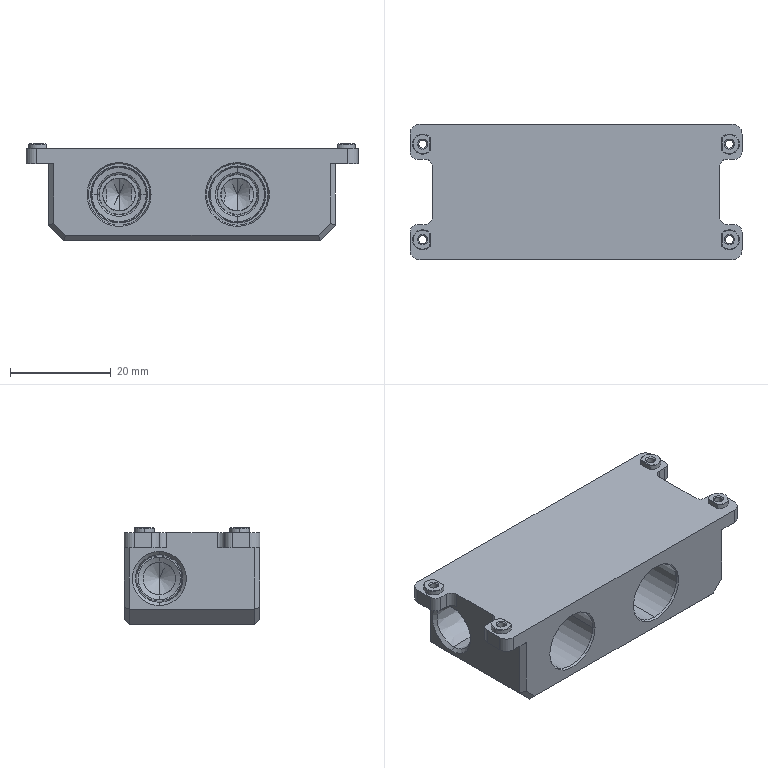NC program | NX | posted with a generic post | part box 66 x 27 x 19.25 mm
Lines 4327 to 5134 of 6448:
(DRILLING_1 , TOOL : D3倒角刀)
N8598 T05 M6
N8600 G54
N8602 G17 G0 G90 X-6.5 Y9.125 S2000 M3
N8604 G43 Z15.5 H5
N8606 G94 G81 G99 Z-5.5 F200. R-1.5
N8608 G80
N8610 G0 X-6.5 Y9.125 Z15.5
N8612 M5
(DRILLING_6 , TOOL : D6.5钻头)
N8614 T09 M6
N8616 G54
N8618 G17 G0 G90 X-6.5 Y9.125 S2000 M3
N8620 G43 Z15.5 H9
N8622 G94 G81 G98 Z-50.5 F200. R-1.5
N8624 G80
N8626 G0 X-6.5 Y9.125 Z15.5
N8628 M5
(DRILLING_2 , TOOL : D8.4钻头)
N8630 T10 M6
N8632 G54
N8634 G17 G0 G90 X-6.5 Y9.125 S1600 M3
N8636 G43 Z15.5 H10
N8638 G94 G83 G98 Z-16.5 F200. Q3. R-1.5
N8640 G80
N8642 G0 X-6.5 Y9.125 Z15.5
N8644 M5
(PLANAR_MILL_4 , TOOL : D3倒角刀)
N8646 T05 M6
N8648 G54
N8650 G17 G0 G90 X-7.5 Y6.038 S4500 M3
N8652 G43 Z15.5 H5
N8654 Z-3.5
N8656 G94 G1 Z-5.5 F600.
N8658 Y5.88
N8660 G3 X-6.5 Y4.88 R1.
N8662 X-2.255 Y9.125 R4.245
N8664 X-6.5 Y4.88 R-4.245
N8666 X-5.5 Y5.88 R1.
N8668 G1 Y6.038
N8670 Z-3.5
N8672 G0 Z15.5
N8674 M5
(THREAD_MILLING , TOOL : NPT)
N8676 T11 M6
N8678 G54
N8680 G17 G0 G90 X-6.5 Y9.125 S4500 M3
N8682 G43 Z15.5 H11
N8684 Z-11.547
N8686 G41 G94 G1 X-6.024 Y8.972 F300. D11
N8688 G3 X-5.595 Y9.555 Z-11.42 R0.412
N8690 X-6.143 Y10.065 Z-11.31 R1.003
N8692 X-6.895 Y10.053 Z-11.199 R1.008
N8694 X-7.43 Y9.524 Z-11.089 R1.01
N8696 X-7.45 Y8.767 Z-10.978 R1.014
N8698 X-6.94 Y8.206 Z-10.868 R1.017
N8700 X-6.18 Y8.154 Z-10.758 R1.021
N8702 X-5.594 Y8.644 Z-10.648 R1.024
N8704 X-5.51 Y9.407 Z-10.537 R1.028
N8706 X-5.979 Y10.017 Z-10.427 R1.031
N8708 X-6.742 Y10.133 Z-10.316 R1.035
N8710 X-7.375 Y9.687 Z-10.206 R1.037
N8712 X-7.524 Y8.924 Z-10.095 R1.042
N8714 X-7.102 Y8.268 Z-9.985 R1.044
N8716 X-6.34 Y8.087 Z-9.875 R1.049
N8718 X-5.664 Y8.484 Z-9.765 R1.051
N8720 X-5.45 Y9.242 Z-9.654 R1.056
N8722 X-5.821 Y9.939 Z-9.544 R1.058
N8724 X-6.574 Y10.186 Z-9.433 R1.063
N8726 X-7.29 Y9.842 Z-9.323 R1.065
N8728 X-7.57 Y9.095 Z-9.212 R1.07
N8730 X-7.254 Y8.36 Z-9.102 R1.072
N8732 X-6.514 Y8.047 Z-8.992 R1.077
N8734 X-5.762 Y8.335 Z-8.882 R1.079
N8736 X-5.417 Y9.066 Z-8.771 R1.083
N8738 X-5.674 Y9.834 Z-8.661 R1.086
N8740 X-6.395 Y10.211 Z-8.55 R1.09
N8742 X-7.178 Y9.985 Z-8.44 R1.093
N8744 X-7.588 Y9.276 Z-8.329 R1.097
N8746 X-7.393 Y8.479 Z-8.219 R1.1
N8748 X-6.697 Y8.037 Z-8.109 R1.104
N8750 X-5.888 Y8.201 Z-7.998 R1.106
N8752 X-5.415 Y8.881 Z-7.888 R1.111
N8754 X-5.545 Y9.702 Z-7.778 R1.113
N8756 X-6.21 Y10.206 Z-7.667 R1.118
N8758 X-7.04 Y10.109 Z-7.557 R1.12
N8760 X-7.574 Y9.462 Z-7.446 R1.125
N8762 X-7.512 Y8.623 Z-7.336 R1.127
N8764 X-6.884 Y8.059 Z-7.226 R1.132
N8766 X-6.038 Y8.087 Z-7.115 R1.134
N8768 X-5.444 Y8.695 Z-7.005 R1.139
N8770 X-5.437 Y9.546 Z-6.895 R1.141
N8772 X-6.024 Y10.168 Z-6.784 R1.145
N8774 X-6.879 Y10.211 Z-6.674 R1.148
N8776 X-7.529 Y9.647 Z-6.563 R1.152
N8778 X-7.607 Y8.789 Z-6.453 R1.155
N8780 X-7.068 Y8.113 Z-6.343 R1.159
N8782 X-6.209 Y7.998 Z-6.232 R1.162
N8784 X-5.507 Y8.512 Z-6.122 R1.166
N8786 X-5.355 Y9.371 Z-6.012 R1.169
N8788 X-5.842 Y10.098 Z-5.901 R1.173
N8790 X-6.699 Y10.286 Z-5.791 R1.175
N8792 X-7.45 Y9.827 Z-5.68 R1.18
N8794 X-7.675 Y8.973 Z-5.57 R1.182
N8796 X-7.245 Y8.199 Z-5.46 R1.187
N8798 X-6.397 Y7.938 Z-5.349 R1.189
N8800 X-5.601 Y8.338 Z-5.239 R1.194
N8802 X-5.303 Y9.179 Z-5.129 R1.196
N8804 X-5.672 Y9.996 Z-5.018 R1.201
N8806 X-6.505 Y10.33 Z-4.908 R1.203
N8808 X-7.34 Y9.994 Z-4.797 R1.208
N8810 X-7.711 Y9.171 Z-4.687 R1.21
N8812 X-7.408 Y8.317 Z-4.577 R1.214
N8814 X-6.597 Y7.91 Z-4.466 R1.217
N8816 X-5.726 Y8.179 Z-4.356 R1.221
N8818 X-5.283 Y8.977 Z-4.246 R1.224
N8820 X-5.517 Y9.863 Z-4.135 R1.228
N8822 X-6.504 Y9.625 Z-3.983 R0.552
N8824 G40
N8826 G1 X-6.5 Y9.125
N8828 G0 Z-11.563
N8830 G41 G1 X-6.045 Y8.918
N8832 G3 X-5.467 Y9.616 Z-11.42 R0.501
N8834 X-6.093 Y10.197 Z-11.31 R1.145
N8836 X-6.95 Y10.184 Z-11.199 R1.149
N8838 X-7.561 Y9.579 Z-11.089 R1.152
N8840 X-7.583 Y8.717 Z-10.978 R1.156
N8842 X-7.001 Y8.078 Z-10.868 R1.159
N8844 X-6.135 Y8.019 Z-10.758 R1.163
N8846 X-5.468 Y8.578 Z-10.648 R1.165
N8848 X-5.374 Y9.446 Z-10.537 R1.17
N8850 X-5.907 Y10.139 Z-10.427 R1.172
N8852 X-6.775 Y10.271 Z-10.316 R1.177
N8854 X-7.494 Y9.763 Z-10.206 R1.179
N8856 X-7.663 Y8.896 Z-10.095 R1.184
N8858 X-7.183 Y8.152 Z-9.985 R1.186
N8860 X-6.319 Y7.947 Z-9.875 R1.191
N8862 X-5.551 Y8.398 Z-9.765 R1.193
N8864 X-5.309 Y9.258 Z-9.654 R1.198
N8866 X-5.73 Y10.048 Z-9.544 R1.2
N8868 X-6.584 Y10.328 Z-9.433 R1.205
N8870 X-7.396 Y9.937 Z-9.323 R1.207
N8872 X-7.712 Y9.091 Z-9.212 R1.211
N8874 X-7.354 Y8.259 Z-9.102 R1.214
N8876 X-6.516 Y7.906 Z-8.992 R1.218
N8878 X-5.665 Y8.231 Z-8.881 R1.221
N8880 X-5.275 Y9.058 Z-8.771 R1.225
N8882 X-5.567 Y9.926 Z-8.661 R1.228
N8884 X-6.381 Y10.353 Z-8.55 R1.232
N8886 X-7.266 Y10.096 Z-8.44 R1.234
N8888 X-7.728 Y9.295 Z-8.329 R1.239
N8890 X-7.507 Y8.396 Z-8.219 R1.241
N8892 X-6.722 Y7.898 Z-8.109 R1.246
N8894 X-5.809 Y8.082 Z-7.998 R1.248
N8896 X-5.276 Y8.85 Z-7.888 R1.253
N8898 X-5.424 Y9.775 Z-7.778 R1.255
N8900 X-6.173 Y10.343 Z-7.667 R1.26
N8902 X-7.108 Y10.233 Z-7.557 R1.262
N8904 X-7.71 Y9.504 Z-7.446 R1.267
N8906 X-7.639 Y8.56 Z-7.336 R1.269
N8908 X-6.932 Y7.926 Z-7.226 R1.274
N8910 X-5.98 Y7.957 Z-7.115 R1.276
N8912 X-5.313 Y8.641 Z-7.005 R1.28
N8914 X-5.305 Y9.599 Z-6.895 R1.283
N8916 X-5.965 Y10.297 Z-6.784 R1.287
N8918 X-6.926 Y10.345 Z-6.674 R1.29
N8920 X-7.655 Y9.712 Z-6.563 R1.294
N8922 X-7.743 Y8.748 Z-6.453 R1.297
N8924 X-7.137 Y7.989 Z-6.343 R1.301
N8926 X-6.173 Y7.861 Z-6.232 R1.303
N8928 X-5.386 Y8.437 Z-6.122 R1.308
N8930 X-5.217 Y9.4 Z-6.012 R1.31
N8932 X-5.763 Y10.215 Z-5.901 R1.315
N8934 X-6.723 Y10.426 Z-5.791 R1.317
N8936 X-7.564 Y9.911 Z-5.68 R1.322
N8938 X-7.816 Y8.955 Z-5.57 R1.324
N8940 X-7.334 Y8.089 Z-5.46 R1.329
N8942 X-6.384 Y7.797 Z-5.349 R1.331
N8944 X-5.494 Y8.245 Z-5.239 R1.336
N8946 X-5.161 Y9.186 Z-5.129 R1.338
N8948 X-5.574 Y10.098 Z-5.018 R1.342
N8950 X-6.505 Y10.472 Z-4.908 R1.345
N8952 X-7.439 Y10.096 Z-4.797 R1.349
N8954 X-7.853 Y9.176 Z-4.687 R1.352
N8956 X-7.514 Y8.223 Z-4.577 R1.356
N8958 X-6.608 Y7.768 Z-4.466 R1.359
N8960 X-5.636 Y8.069 Z-4.356 R1.363
N8962 X-5.142 Y8.96 Z-4.246 R1.366
N8964 X-5.404 Y9.949 Z-4.135 R1.37
N8966 X-6.545 Y9.623 Z-3.973 R0.635
N8968 G40
N8970 G1 X-6.5 Y9.125
N8972 G0 Z-11.574
N8974 G41 G1 X-6.066 Y8.877
N8976 G3 X-5.339 Y9.676 Z-11.42 R0.585
N8978 X-6.042 Y10.33 Z-11.31 R1.287
N8980 X-7.005 Y10.314 Z-11.199 R1.291
N8982 X-7.691 Y9.635 Z-11.089 R1.293
N8984 X-7.716 Y8.667 Z-10.978 R1.298
N8986 X-7.062 Y7.95 Z-10.868 R1.3
N8988 X-6.091 Y7.885 Z-10.758 R1.305
N8990 X-5.343 Y8.511 Z-10.648 R1.307
N8992 X-5.237 Y9.484 Z-10.537 R1.312
N8994 X-5.835 Y10.261 Z-10.427 R1.314
N8996 X-6.808 Y10.408 Z-10.316 R1.319
N8998 X-7.614 Y9.84 Z-10.206 R1.321
N9000 X-7.802 Y8.869 Z-10.095 R1.326
N9002 X-7.264 Y8.036 Z-9.985 R1.328
N9004 X-6.297 Y7.807 Z-9.875 R1.333
N9006 X-5.439 Y8.312 Z-9.765 R1.335
N9008 X-5.168 Y9.274 Z-9.654 R1.339
N9010 X-5.639 Y10.157 Z-9.544 R1.342
N9012 X-6.594 Y10.469 Z-9.433 R1.346
N9014 X-7.501 Y10.033 Z-9.323 R1.349
N9016 X-7.854 Y9.087 Z-9.212 R1.353
N9018 X-7.453 Y8.158 Z-9.102 R1.356
N9020 X-6.518 Y7.764 Z-8.992 R1.36
N9022 X-5.569 Y8.127 Z-8.881 R1.362
N9024 X-5.134 Y9.05 Z-8.771 R1.367
N9026 X-5.459 Y10.019 Z-8.661 R1.369
N9028 X-6.368 Y10.494 Z-8.55 R1.374
N9030 X-7.354 Y10.207 Z-8.44 R1.376
N9032 X-7.869 Y9.315 Z-8.329 R1.381
N9034 X-7.622 Y8.313 Z-8.219 R1.383
N9036 X-6.748 Y7.758 Z-8.109 R1.388
N9038 X-5.731 Y7.964 Z-7.998 R1.39
N9040 X-5.138 Y8.819 Z-7.888 R1.395
N9042 X-5.302 Y9.849 Z-7.778 R1.397
N9044 X-6.136 Y10.48 Z-7.667 R1.402
N9046 X-7.177 Y10.358 Z-7.557 R1.404
N9048 X-7.845 Y9.547 Z-7.446 R1.408
N9050 X-7.766 Y8.497 Z-7.336 R1.411
N9052 X-6.98 Y7.792 Z-7.226 R1.415
N9054 X-5.922 Y7.828 Z-7.115 R1.418
N9056 X-5.182 Y8.588 Z-7.005 R1.422
N9058 X-5.174 Y9.651 Z-6.895 R1.425
N9060 X-5.906 Y10.426 Z-6.784 R1.429
N9062 X-6.973 Y10.479 Z-6.674 R1.431
N9064 X-7.781 Y9.776 Z-6.563 R1.436
N9066 X-7.879 Y8.707 Z-6.453 R1.438
N9068 X-7.207 Y7.866 Z-6.343 R1.443
N9070 X-6.138 Y7.724 Z-6.232 R1.445
N9072 X-5.265 Y8.363 Z-6.122 R1.45
N9074 X-5.078 Y9.43 Z-6.012 R1.452
N9076 X-5.684 Y10.333 Z-5.901 R1.457
N9078 X-6.747 Y10.565 Z-5.791 R1.459
N9080 X-7.678 Y9.995 Z-5.68 R1.464
N9082 X-7.956 Y8.937 Z-5.57 R1.466
N9084 X-7.422 Y7.978 Z-5.46 R1.471
N9086 X-6.372 Y7.655 Z-5.349 R1.473
N9088 X-5.387 Y8.151 Z-5.239 R1.477
N9090 X-5.019 Y9.192 Z-5.129 R1.48
N9092 X-5.476 Y10.201 Z-5.018 R1.484
N9094 X-6.506 Y10.614 Z-4.908 R1.487
N9096 X-7.538 Y10.198 Z-4.797 R1.491
N9098 X-7.995 Y9.181 Z-4.687 R1.494
N9100 X-7.62 Y8.128 Z-4.577 R1.498
N9102 X-6.619 Y7.627 Z-4.466 R1.5
N9104 X-5.546 Y7.959 Z-4.356 R1.505
N9106 X-5.001 Y8.943 Z-4.246 R1.507
N9108 X-5.29 Y10.034 Z-4.135 R1.512
N9110 X-6.578 Y9.619 Z-3.965 R0.715
N9112 G40
N9114 G1 X-6.5 Y9.125
N9116 G0 Z-11.574
N9118 G41 G1 X-6.066 Y8.877
N9120 G3 X-5.339 Y9.676 Z-11.42 R0.585
N9122 X-6.042 Y10.33 Z-11.31 R1.287
N9124 X-7.005 Y10.314 Z-11.199 R1.291
N9126 X-7.691 Y9.635 Z-11.089 R1.293
N9128 X-7.716 Y8.667 Z-10.978 R1.298
N9130 X-7.062 Y7.95 Z-10.868 R1.3
N9132 X-6.091 Y7.885 Z-10.758 R1.305
N9134 X-5.343 Y8.511 Z-10.648 R1.307
N9136 X-5.237 Y9.484 Z-10.537 R1.312
N9138 X-5.835 Y10.261 Z-10.427 R1.314
N9140 X-6.808 Y10.408 Z-10.316 R1.319
N9142 X-7.614 Y9.84 Z-10.206 R1.321
N9144 X-7.802 Y8.869 Z-10.095 R1.326
N9146 X-7.264 Y8.036 Z-9.985 R1.328
N9148 X-6.297 Y7.807 Z-9.875 R1.333
N9150 X-5.439 Y8.312 Z-9.765 R1.335
N9152 X-5.168 Y9.274 Z-9.654 R1.339
N9154 X-5.639 Y10.157 Z-9.544 R1.342
N9156 X-6.594 Y10.469 Z-9.433 R1.346
N9158 X-7.501 Y10.033 Z-9.323 R1.349
N9160 X-7.854 Y9.087 Z-9.212 R1.353
N9162 X-7.453 Y8.158 Z-9.102 R1.356
N9164 X-6.518 Y7.764 Z-8.992 R1.36
N9166 X-5.569 Y8.127 Z-8.881 R1.362
N9168 X-5.134 Y9.05 Z-8.771 R1.367
N9170 X-5.459 Y10.019 Z-8.661 R1.369
N9172 X-6.368 Y10.494 Z-8.55 R1.374
N9174 X-7.354 Y10.207 Z-8.44 R1.376
N9176 X-7.869 Y9.315 Z-8.329 R1.381
N9178 X-7.622 Y8.313 Z-8.219 R1.383
N9180 X-6.748 Y7.758 Z-8.109 R1.388
N9182 X-5.731 Y7.964 Z-7.998 R1.39
N9184 X-5.138 Y8.819 Z-7.888 R1.395
N9186 X-5.302 Y9.849 Z-7.778 R1.397
N9188 X-6.136 Y10.48 Z-7.667 R1.402
N9190 X-7.177 Y10.358 Z-7.557 R1.404
N9192 X-7.845 Y9.547 Z-7.446 R1.408
N9194 X-7.766 Y8.497 Z-7.336 R1.411
N9196 X-6.98 Y7.792 Z-7.226 R1.415
N9198 X-5.922 Y7.828 Z-7.115 R1.418
N9200 X-5.182 Y8.588 Z-7.005 R1.422
N9202 X-5.174 Y9.651 Z-6.895 R1.425
N9204 X-5.906 Y10.426 Z-6.784 R1.429
N9206 X-6.973 Y10.479 Z-6.674 R1.431
N9208 X-7.781 Y9.776 Z-6.563 R1.436
N9210 X-7.879 Y8.707 Z-6.453 R1.438
N9212 X-7.207 Y7.866 Z-6.343 R1.443
N9214 X-6.138 Y7.724 Z-6.232 R1.445
N9216 X-5.265 Y8.363 Z-6.122 R1.45
N9218 X-5.078 Y9.43 Z-6.012 R1.452
N9220 X-5.684 Y10.333 Z-5.901 R1.457
N9222 X-6.747 Y10.565 Z-5.791 R1.459
N9224 X-7.678 Y9.995 Z-5.68 R1.464
N9226 X-7.956 Y8.937 Z-5.57 R1.466
N9228 X-7.422 Y7.978 Z-5.46 R1.471
N9230 X-6.372 Y7.655 Z-5.349 R1.473
N9232 X-5.387 Y8.151 Z-5.239 R1.477
N9234 X-5.019 Y9.192 Z-5.129 R1.48
N9236 X-5.476 Y10.201 Z-5.018 R1.484
N9238 X-6.506 Y10.614 Z-4.908 R1.487
N9240 X-7.538 Y10.198 Z-4.797 R1.491
N9242 X-7.995 Y9.181 Z-4.687 R1.494
N9244 X-7.62 Y8.128 Z-4.577 R1.498
N9246 X-6.619 Y7.627 Z-4.466 R1.5
N9248 X-5.546 Y7.959 Z-4.356 R1.505
N9250 X-5.001 Y8.943 Z-4.246 R1.507
N9252 X-5.29 Y10.034 Z-4.135 R1.512
N9254 X-6.578 Y9.619 Z-3.965 R0.715
N9256 G40
N9258 G1 X-6.5 Y9.125
N9260 G0 Z-11.574
N9262 G41 G1 X-6.066 Y8.877
N9264 G3 X-5.339 Y9.676 Z-11.42 R0.585
N9266 X-6.042 Y10.33 Z-11.31 R1.287
N9268 X-7.005 Y10.314 Z-11.199 R1.291
N9270 X-7.691 Y9.635 Z-11.089 R1.293
N9272 X-7.716 Y8.667 Z-10.978 R1.298
N9274 X-7.062 Y7.95 Z-10.868 R1.3
N9276 X-6.091 Y7.885 Z-10.758 R1.305
N9278 X-5.343 Y8.511 Z-10.648 R1.307
N9280 X-5.237 Y9.484 Z-10.537 R1.312
N9282 X-5.835 Y10.261 Z-10.427 R1.314
N9284 X-6.808 Y10.408 Z-10.316 R1.319
N9286 X-7.614 Y9.84 Z-10.206 R1.321
N9288 X-7.802 Y8.869 Z-10.095 R1.326
N9290 X-7.264 Y8.036 Z-9.985 R1.328
N9292 X-6.297 Y7.807 Z-9.875 R1.333
N9294 X-5.439 Y8.312 Z-9.765 R1.335
N9296 X-5.168 Y9.274 Z-9.654 R1.339
N9298 X-5.639 Y10.157 Z-9.544 R1.342
N9300 X-6.594 Y10.469 Z-9.433 R1.346
N9302 X-7.501 Y10.033 Z-9.323 R1.349
N9304 X-7.854 Y9.087 Z-9.212 R1.353
N9306 X-7.453 Y8.158 Z-9.102 R1.356
N9308 X-6.518 Y7.764 Z-8.992 R1.36
N9310 X-5.569 Y8.127 Z-8.881 R1.362
N9312 X-5.134 Y9.05 Z-8.771 R1.367
N9314 X-5.459 Y10.019 Z-8.661 R1.369
N9316 X-6.368 Y10.494 Z-8.55 R1.374
N9318 X-7.354 Y10.207 Z-8.44 R1.376
N9320 X-7.869 Y9.315 Z-8.329 R1.381
N9322 X-7.622 Y8.313 Z-8.219 R1.383
N9324 X-6.748 Y7.758 Z-8.109 R1.388
N9326 X-5.731 Y7.964 Z-7.998 R1.39
N9328 X-5.138 Y8.819 Z-7.888 R1.395
N9330 X-5.302 Y9.849 Z-7.778 R1.397
N9332 X-6.136 Y10.48 Z-7.667 R1.402
N9334 X-7.177 Y10.358 Z-7.557 R1.404
N9336 X-7.845 Y9.547 Z-7.446 R1.408
N9338 X-7.766 Y8.497 Z-7.336 R1.411
N9340 X-6.98 Y7.792 Z-7.226 R1.415
N9342 X-5.922 Y7.828 Z-7.115 R1.418
N9344 X-5.182 Y8.588 Z-7.005 R1.422
N9346 X-5.174 Y9.651 Z-6.895 R1.425
N9348 X-5.906 Y10.426 Z-6.784 R1.429
N9350 X-6.973 Y10.479 Z-6.674 R1.431
N9352 X-7.781 Y9.776 Z-6.563 R1.436
N9354 X-7.879 Y8.707 Z-6.453 R1.438
N9356 X-7.207 Y7.866 Z-6.343 R1.443
N9358 X-6.138 Y7.724 Z-6.232 R1.445
N9360 X-5.265 Y8.363 Z-6.122 R1.45
N9362 X-5.078 Y9.43 Z-6.012 R1.452
N9364 X-5.684 Y10.333 Z-5.901 R1.457
N9366 X-6.747 Y10.565 Z-5.791 R1.459
N9368 X-7.678 Y9.995 Z-5.68 R1.464
N9370 X-7.956 Y8.937 Z-5.57 R1.466
N9372 X-7.422 Y7.978 Z-5.46 R1.471
N9374 X-6.372 Y7.655 Z-5.349 R1.473
N9376 X-5.387 Y8.151 Z-5.239 R1.477
N9378 X-5.019 Y9.192 Z-5.129 R1.48
N9380 X-5.476 Y10.201 Z-5.018 R1.484
N9382 X-6.506 Y10.614 Z-4.908 R1.487
N9384 X-7.538 Y10.198 Z-4.797 R1.491
N9386 X-7.995 Y9.181 Z-4.687 R1.494
N9388 X-7.62 Y8.128 Z-4.577 R1.498
N9390 X-6.619 Y7.627 Z-4.466 R1.5
N9392 X-5.546 Y7.959 Z-4.356 R1.505
N9394 X-5.001 Y8.943 Z-4.246 R1.507
N9396 X-5.29 Y10.034 Z-4.135 R1.512
N9398 X-6.578 Y9.619 Z-3.965 R0.715
N9400 G40
N9402 G1 X-6.5 Y9.125
N9404 G0 Z15.5
N9406 M5
(FLOOR_WALL_1 , TOOL : D50面刀)
N9408 T01 M6
N9410 G54
N9412 G17 G0 G90 X76. Y6.5 S4500 M3
N9414 G43 Z20. H1
N9416 Z8.008
N9418 G94 G1 Z5.008 F1500.
N9420 X73.
N9422 X-73.
N9424 X-76.
N9426 Z8.008
N9428 G0 Z20.
N9430 X76.
N9432 Z7.017
N9434 G1 Z4.017
N9436 X73.
N9438 X-73.
N9440 X-76.
N9442 Z7.017
N9444 G0 Z20.
N9446 X76.
N9448 Z6.025
N9450 G1 Z3.025
N9452 X73.
N9454 X-73.
N9456 X-76.
N9458 Z6.025
N9460 G0 Z20.
N9462 X76.
N9464 Z5.033
N9466 G1 Z2.033
N9468 X73.
N9470 X-73.
N9472 X-76.
N9474 Z5.033
N9476 G0 Z20.
N9478 X76.
N9480 Z4.042
N9482 G1 Z1.042
N9484 X73.
N9486 X-73.
N9488 X-76.
N9490 Z4.042
N9492 G0 Z20.
N9494 X76.
N9496 Z3.05
N9498 G1 Z0.05
N9500 X73.
N9502 X-73.
N9504 X-76.
N9506 Z3.05
N9508 G0 Z20.
(FLOOR_WALL_1_COPY , TOOL : D50面刀)
N9510 X76.
N9512 Z3.
N9514 G1 Z0. F600.
N9516 X73.
N9518 X-73.
N9520 X-76.
N9522 Z3.
N9524 G0 Z20.
N9526 M5
(FLOOR_WALL_2 , TOOL : D8开粗)
N9528 T02 M6
N9530 G54
N9532 G17 G0 G90 X-2. Y20.5 S6500 M3
N9534 G43 Z20. H2
N9536 Z2.1
N9538 G94 G1 Z-0.9 F1000.
N9540 Y19.
N9542 G3 X0. Y17. R2.
N9544 G1 X31.
N9546 G2 X36.5 Y11.5 R5.5
N9548 G1 Y10.6
N9550 G3 X25.925 Y13.535 R6.1
N9552 G1 X24.9 Y12.373
N9554 Y6.627
N9556 X25.925 Y5.465
N9558 G3 X36.5 Y8.4 R6.1
N9560 G1 Y8.
N9562 G2 X32.409 Y3.083 R5.
N9564 G1 X32. Y3.008
N9566 Y-3.008
N9568 X32.409 Y-3.083
N9570 G2 X36.5 Y-8. R5.
N9572 G1 Y-8.4
N9574 G3 X25.925 Y-5.465 R6.1
N9576 G1 X24.9 Y-6.627
N9578 Y-12.373
N9580 X25.925 Y-13.535
N9582 G3 X36.5 Y-10.6 R6.1
N9584 G1 Y-11.5
N9586 G2 X31. Y-17. R5.5
N9588 G1 X-31.
N9590 G2 X-36.5 Y-11.5 R5.5
N9592 G1 Y-10.6
N9594 G3 X-25.925 Y-13.535 R6.1
N9596 G1 X-24.9 Y-12.373
N9598 Y-6.627
N9600 X-25.925 Y-5.465
N9602 G3 X-36.5 Y-8.4 R6.1
N9604 G1 Y-7.999
N9606 G2 X-32.409 Y-3.083 R5.
N9608 G1 X-32. Y-3.008
N9610 Y3.008
N9612 X-32.409 Y3.083
N9614 G2 X-36.5 Y8. R5.
N9616 G1 Y8.4
N9618 G3 X-25.925 Y5.465 R6.1
N9620 G1 X-24.9 Y6.627
N9622 Y12.373
N9624 X-25.925 Y13.535
N9626 G3 X-36.5 Y10.6 R6.1
N9628 G1 Y11.5
N9630 G2 X-31. Y17. R5.5
N9632 G1 X0.
N9634 Y11.
N9636 X18.9
N9638 Y6.627
N9640 G3 X20.4 Y2.659 R6.
N9642 G1 X21.425 Y1.497
N9644 G3 X23.006 Y0. R12.1
N9646 G1 X27.028
N9648 X23.006
N9650 G3 X21.425 Y-1.497 R12.1
N9652 G1 X20.4 Y-2.659
N9654 G3 X18.9 Y-6.627 R6.
N9656 G1 Y-11.
N9658 X-18.9
N9660 Y-6.627
N9662 G3 X-20.4 Y-2.659 R6.
N9664 G1 X-21.425 Y-1.497
N9666 G3 X-23.006 Y0. R12.1
N9668 G1 X-27.028
N9670 X-23.006
N9672 G3 X-21.425 Y1.497 R12.1
N9674 G1 X-20.4 Y2.659
N9676 G3 X-18.9 Y6.627 R6.
N9678 G1 Y11.
N9680 X0.
N9682 Y5.
N9684 X13.011
N9686 G3 X14.896 Y0. R12.
N9688 X13.011 Y-5. R12.
N9690 G1 X-13.011
N9692 G3 X-14.896 Y0. R12.
N9694 X-13.011 Y5. R12.
N9696 G1 X0.
N9698 Y1.4
N9700 X10.202
N9702 G3 X10.778 Y0. R15.6
N9704 X10.202 Y-1.4 R15.6
N9706 G1 X-10.202
N9708 G3 X-10.778 Y0. R15.6
N9710 X-10.202 Y1.4 R15.6
N9712 G1 X0.
N9714 X1.
N9716 G3 X3. Y3.4 R2.
N9718 G1 Z2.1
N9720 G0 Z20.
N9722 M5
(FLOOR_WALL_2_COPY , TOOL : D8精光)
N9724 T03 M6
N9726 G54
N9728 G17 G0 G90 X-2. Y20.5 S6500 M3
N9730 G43 Z20. H3
N9732 Z2.
N9734 G94 G1 Z-1. F600.
N9736 Y19.
N9738 G3 X0. Y17. R2.
N9740 G1 X31.
N9742 G2 X36.5 Y11.5 R5.5
N9744 G1 Y9.5
N9746 G3 X26. Y13.469 R6.
N9748 G1 X25. Y12.335
N9750 Y6.665
N9752 X26. Y5.531
N9754 G3 X36.5 Y9.5 R6.
N9756 G1 Y8.
N9758 G2 X32.409 Y3.083 R5.
N9760 G1 X32. Y3.008
N9762 Y-3.008
N9764 X32.409 Y-3.083
N9766 G2 X36.5 Y-8. R5.
N9768 G1 Y-9.5
N9770 G3 X26. Y-5.531 R6.
N9772 G1 X25. Y-6.665
N9774 Y-12.335
N9776 X26. Y-13.469
N9778 G3 X36.5 Y-9.5 R6.
N9780 G1 Y-11.5
N9782 G2 X31. Y-17. R5.5
N9784 G1 X-31.
N9786 G2 X-36.5 Y-11.5 R5.5
N9788 G1 Y-9.501
N9790 G3 X-26. Y-13.469 R6.
N9792 G1 X-25. Y-12.335
N9794 Y-6.665
N9796 X-26. Y-5.531
N9798 G3 X-36.5 Y-9.499 R6.
N9800 G1 Y-7.999
N9802 G2 X-32.409 Y-3.083 R5.
N9804 G1 X-32. Y-3.008
N9806 Y3.008
N9808 X-32.409 Y3.083
N9810 G2 X-36.5 Y8. R5.
N9812 G1 Y9.499
N9814 G3 X-26. Y5.531 R6.
N9816 G1 X-25. Y6.665
N9818 Y12.335
N9820 X-26. Y13.469
N9822 G3 X-36.5 Y9.501 R6.
N9824 G1 Y11.5
N9826 G2 X-31. Y17. R5.5
N9828 G1 X0.
N9830 Y11.
N9832 X19.
N9834 Y6.665
N9836 G3 X20.5 Y2.697 R6.
N9838 G1 X21.5 Y1.563
N9840 G3 X23.169 Y0. R12.
N9842 G1 X27.238
N9844 X23.169
N9846 G3 X21.5 Y-1.563 R12.
N9848 G1 X20.5 Y-2.697
N9850 G3 X19. Y-6.665 R6.
N9852 G1 Y-11.
N9854 X-19.
N9856 Y-6.665
N9858 G3 X-20.5 Y-2.697 R6.
N9860 G1 X-21.5 Y-1.563
N9862 G3 X-23.169 Y0. R12.
N9864 G1 X-27.238
N9866 X-23.169
N9868 G3 X-21.5 Y1.563 R12.
N9870 G1 X-20.5 Y2.697
N9872 G3 X-19. Y6.665 R6.
N9874 G1 Y11.
N9876 X0.
N9878 Y5.
N9880 X13.116
N9882 G3 X15.021 Y0. R12.
N9884 X13.116 Y-5. R12.
N9886 G1 X-13.116
N9888 G3 X-15.021 Y0. R12.
N9890 X-13.116 Y5. R12.
N9892 G1 X0.
N9894 Y1.4
N9896 X10.315
N9898 G3 X10.896 Y0. R15.6
N9900 X10.315 Y-1.4 R15.6
N9902 G1 X-10.315
N9904 G3 X-10.896 Y0. R15.6
N9906 X-10.315 Y1.4 R15.6
N9908 G1 X0.
N9910 X1.
N9912 G3 X3. Y3.4 R2.
N9914 G1 Z2.
N9916 G0 Z20.
N9918 M5
(DRILLING_3 , TOOL : D3倒角刀)
N9920 T05 M6
N9922 G54
N9924 G17 G0 G90 X30.5 Y-9.5 S3000 M3
N9926 G43 Z20. H5
N9928 G94 G81 G99 Z-1. F250. R3.
N9930 X-30.5
N9932 Y9.5
N9934 X30.5
N9936 G80
N9938 G0 X30.5 Y9.5 Z20.
(PLANAR_MILL_3_COPY , TOOL : D3倒角刀)
N9940 X-27.8 Y10. S4500
N9942 Z1.3
N9944 G1 Z-0.7 F800.
N9946 G3 X-28.3 Y9.5 R0.5
N9948 G1 Y8.177
N9950 G2 X-28.475 Y7.714 R0.7
N9952 X-28.475 Y11.286 R-2.7
N9954 X-28.3 Y10.823 R0.7
N9956 G1 Y9.5
N9958 G3 X-27.8 Y9. R0.5
N9960 G1 Z1.3
N9962 G0 Z20.
N9964 Y-9.
N9966 Z1.3
N9968 G1 Z-0.7
N9970 G3 X-28.3 Y-9.5 R0.5
N9972 G1 Y-10.823
N9974 G2 X-28.475 Y-11.286 R0.7
N9976 X-28.475 Y-7.714 R-2.7
N9978 X-28.3 Y-8.177 R0.7
N9980 G1 Y-9.5
N9982 G3 X-27.8 Y-10. R0.5
N9984 G1 Z1.3
N9986 G0 Z20.
N9988 X27.8
N9990 Z1.3
N9992 G1 Z-0.7
N9994 G3 X28.3 Y-9.5 R0.5
N9996 G1 Y-8.177
N9998 G2 X28.475 Y-7.714 R0.7
N10000 X28.475 Y-11.286 R-2.7
N10002 X28.3 Y-10.823 R0.7
N10004 G1 Y-9.5
N10006 G3 X27.8 Y-9. R0.5
N10008 G1 Z1.3
N10010 G0 Z20.
N10012 Y9.
N10014 Z1.3
N10016 G1 Z-0.7
N10018 G3 X28.3 Y9.5 R0.5
N10020 G1 Y10.823
N10022 G2 X28.475 Y11.286 R0.7
N10024 X28.475 Y7.714 R-2.7
N10026 X28.3 Y8.177 R0.7
N10028 G1 Y9.5
N10030 G3 X27.8 Y10. R0.5
N10032 G1 Z1.3
N10034 G0 Z20.
(PLANAR_MILL_3 , TOOL : D3倒角刀)
N10036 X-2. Y16.7
N10038 Z-0.2
N10040 G1 Z-2.2
N10042 G3 X0. Y14.7 R2.
N10044 G1 X31.
N10046 G2 X34.2 Y11.5 R3.2
N10048 G1 Y8.
N10050 G2 X31.5 Y5.3 R2.7
N10052 G1 X30.
N10054 G3 X29.7 Y5. R0.3
N10056 G1 Y-5.
N10058 G3 X30. Y-5.3 R0.3
N10060 G1 X31.5
N10062 G2 X34.2 Y-8. R2.7
N10064 G1 Y-11.5
N10066 G2 X31. Y-14.7 R3.2
N10068 G1 X-31.
N10070 G2 X-34.2 Y-11.5 R3.2
N10072 G1 Y-8.
N10074 G2 X-31.5 Y-5.3 R2.7
N10076 G1 X-30.
N10078 G3 X-29.7 Y-5. R0.3
N10080 G1 Y5.
N10082 G3 X-30. Y5.3 R0.3
N10084 G1 X-31.5
N10086 G2 X-34.2 Y8. R2.7
N10088 G1 Y11.5
N10090 G2 X-31. Y14.7 R3.2
N10092 G1 X0.
N10094 G3 X2. Y16.7 R2.
N10096 G1 Z-0.2
N10098 G0 Z20.
(DRILLING_4 , TOOL : D3倒角刀)
N10100 X-9. Y-9.125 S3000
N10102 G81 Z-1. F250. R3.
N10104 X14.5
N10106 G80
N10108 G0 X14.5 Y-9.125 Z20.
N10110 M5
(DRILLING_4_COPY , TOOL : D6.5钻头)
N10112 T09 M6
N10114 G54
N10116 G17 G0 G90 X-9. Y-9.125 S2000 M3
N10118 G43 Z20. H9
N10120 G94 G83 G99 Z-24.75 F200. Q3. R3.
N10122 X14.5
N10124 G80
N10126 G0 X14.5 Y-9.125 Z20.
N10128 M5